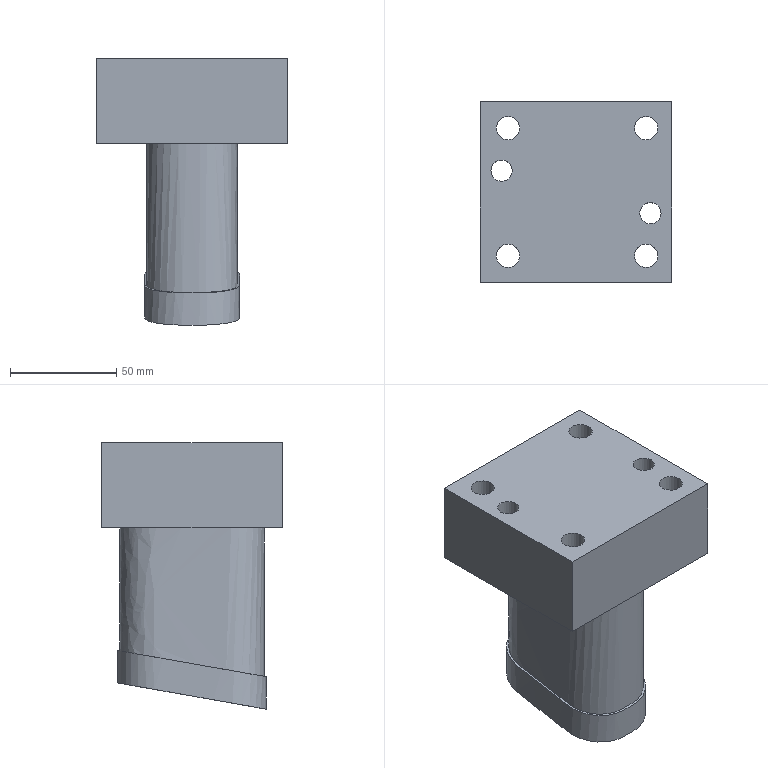Part | NX | features solid 2 | 1 solid | 28 faces | box 90 x 85 x 125.162 mm | volume 481222 mm3 | plane 12 | cylinder 12 | spline 4 | commonest cylinder face diameters 11 x6 17.5 x4 10 x2